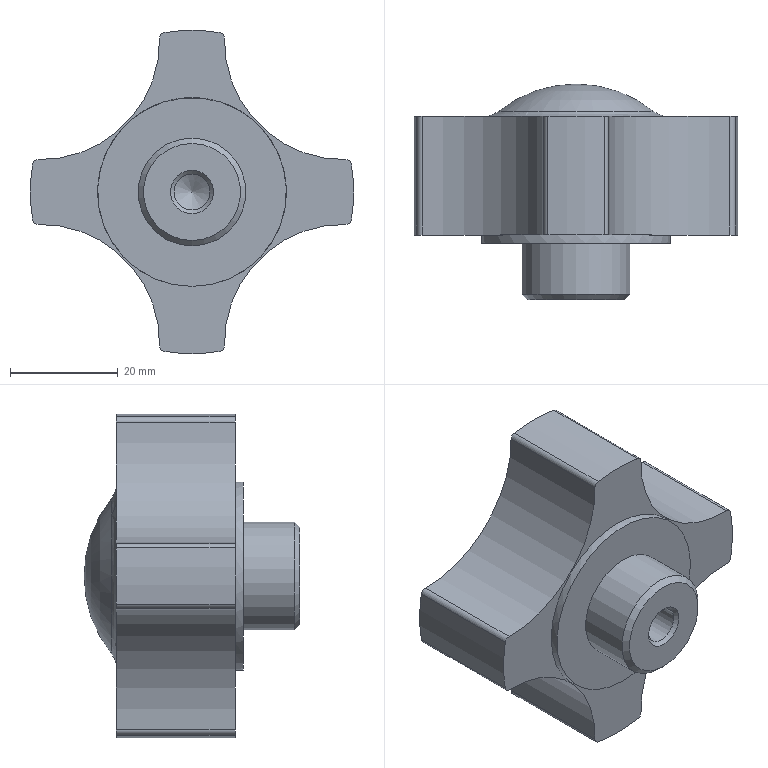Part | STEP file | Superstructure_3 | 1 solid | 28 faces | box 60 x 39.998 x 60 mm | volume 44038 mm3 | cylinder 19 | plane 4 | cone 3 | sphere 1 | torus 1 | commonest cylinder face diameters 2 x8 44 x4 60 x4 6.647 x1 20 x1 35 x1